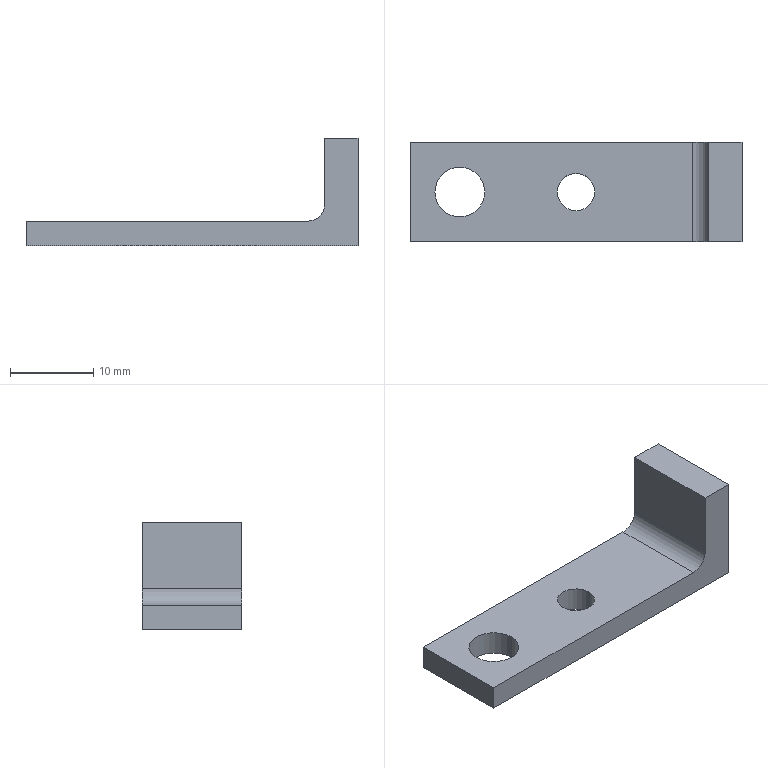Part | SolidWorks | features Extrusion 1, Fillet 1, ICE 1 | 1 solid | 13 faces | box 40 x 12 x 13 mm | volume 1798 mm3 | plane 8 | cylinder 5 | commonest cylinder face diameters 4.5 x2 6 x2 4 x1
STEP:
#1=CARTESIAN_POINT('',(3.,6.,3.));
#2=VERTEX_POINT('',#1);
#3=CARTESIAN_POINT('',(9.,6.,3.));
#4=VERTEX_POINT('',#3);
#5=CARTESIAN_POINT('',(6.,6.,3.));
#6=DIRECTION('',(0.,0.,1.));
#7=DIRECTION('',(1.,0.,0.));
#8=AXIS2_PLACEMENT_3D('',#5,#6,#7);
#9=CIRCLE('',#8,3.);
#10=EDGE_CURVE('',#2,#4,#9,.T.);
#11=ORIENTED_EDGE('',*,*,#10,.T.);
#12=CARTESIAN_POINT('',(9.,6.,0.));
#13=VERTEX_POINT('',#12);
#14=CARTESIAN_POINT('',(9.,6.,3.));
#15=DIRECTION('',(0.,0.,-1.));
#16=VECTOR('',#15,1000.);
#17=LINE('',#14,#16);
#18=EDGE_CURVE('',#4,#13,#17,.T.);
#19=ORIENTED_EDGE('',*,*,#18,.T.);
#20=CARTESIAN_POINT('',(3.,6.,0.));
#21=VERTEX_POINT('',#20);
#22=CARTESIAN_POINT('',(6.,6.,0.));
#23=DIRECTION('',(0.,0.,1.));
#24=DIRECTION('',(1.,0.,0.));
#25=AXIS2_PLACEMENT_3D('',#22,#23,#24);
#26=CIRCLE('',#25,3.);
#27=EDGE_CURVE('',#21,#13,#26,.T.);
#28=ORIENTED_EDGE('',*,*,#27,.F.);
#29=CARTESIAN_POINT('',(3.,6.,3.));
#30=DIRECTION('',(0.,0.,-1.));
#31=VECTOR('',#30,1000.);
#32=LINE('',#29,#31);
#33=EDGE_CURVE('',#2,#21,#32,.T.);
#34=ORIENTED_EDGE('',*,*,#33,.F.);
#35=EDGE_LOOP('',(#11,#19,#28,#34));
#36=FACE_OUTER_BOUND('',#35,.T.);
#37=CARTESIAN_POINT('',(6.,6.,3.));
#38=DIRECTION('',(0.,0.,-1.));
#39=DIRECTION('',(-1.,0.,0.));
#40=AXIS2_PLACEMENT_3D('',#37,#38,#39);
#41=CYLINDRICAL_SURFACE('',#40,3.);
#42=ADVANCED_FACE('',(#36),#41,.F.);
#43=CARTESIAN_POINT('',(17.75,6.,3.));
#44=VERTEX_POINT('',#43);
#45=CARTESIAN_POINT('',(22.25,6.,3.));
#46=VERTEX_POINT('',#45);
#47=CARTESIAN_POINT('',(20.,6.,3.));
#48=DIRECTION('',(0.,0.,1.));
#49=DIRECTION('',(1.,0.,0.));
#50=AXIS2_PLACEMENT_3D('',#47,#48,#49);
#51=CIRCLE('',#50,2.25);
#52=EDGE_CURVE('',#44,#46,#51,.T.);
#53=ORIENTED_EDGE('',*,*,#52,.T.);
#54=CARTESIAN_POINT('',(22.25,6.,0.));
#55=VERTEX_POINT('',#54);
#56=CARTESIAN_POINT('',(22.25,6.,3.));
#57=DIRECTION('',(0.,0.,-1.));
#58=VECTOR('',#57,1000.);
#59=LINE('',#56,#58);
#60=EDGE_CURVE('',#46,#55,#59,.T.);
#61=ORIENTED_EDGE('',*,*,#60,.T.);
#62=CARTESIAN_POINT('',(17.75,6.,0.));
#63=VERTEX_POINT('',#62);
#64=CARTESIAN_POINT('',(20.,6.,0.));
#65=DIRECTION('',(0.,0.,1.));
#66=DIRECTION('',(1.,0.,0.));
#67=AXIS2_PLACEMENT_3D('',#64,#65,#66);
#68=CIRCLE('',#67,2.25);
#69=EDGE_CURVE('',#63,#55,#68,.T.);
#70=ORIENTED_EDGE('',*,*,#69,.F.);
#71=CARTESIAN_POINT('',(17.75,6.,3.));
#72=DIRECTION('',(0.,0.,-1.));
#73=VECTOR('',#72,1000.);
#74=LINE('',#71,#73);
#75=EDGE_CURVE('',#44,#63,#74,.T.);
#76=ORIENTED_EDGE('',*,*,#75,.F.);
#77=EDGE_LOOP('',(#53,#61,#70,#76));
#78=FACE_OUTER_BOUND('',#77,.T.);
#79=CARTESIAN_POINT('',(20.,6.,3.));
#80=DIRECTION('',(0.,0.,-1.));
#81=DIRECTION('',(-1.,0.,0.));
#82=AXIS2_PLACEMENT_3D('',#79,#80,#81);
#83=CYLINDRICAL_SURFACE('',#82,2.25);
#84=ADVANCED_FACE('',(#78),#83,.F.);
#85=ORIENTED_EDGE('',*,*,#10,.F.);
#86=CARTESIAN_POINT('',(6.,6.,3.));
#87=DIRECTION('',(0.,0.,1.));
#88=DIRECTION('',(1.,0.,0.));
#89=AXIS2_PLACEMENT_3D('',#86,#87,#88);
#90=CIRCLE('',#89,3.);
#91=EDGE_CURVE('',#4,#2,#90,.T.);
#92=ORIENTED_EDGE('',*,*,#91,.F.);
#93=EDGE_LOOP('',(#85,#92));
#94=FACE_BOUND('',#93,.T.);
#95=ORIENTED_EDGE('',*,*,#52,.F.);
#96=CARTESIAN_POINT('',(20.,6.,3.));
#97=DIRECTION('',(0.,0.,1.));
#98=DIRECTION('',(1.,0.,0.));
#99=AXIS2_PLACEMENT_3D('',#96,#97,#98);
#100=CIRCLE('',#99,2.25);
#101=EDGE_CURVE('',#46,#44,#100,.T.);
#102=ORIENTED_EDGE('',*,*,#101,.F.);
#103=EDGE_LOOP('',(#95,#102));
#104=FACE_BOUND('',#103,.T.);
#105=CARTESIAN_POINT('',(0.,0.,3.));
#106=VERTEX_POINT('',#105);
#107=CARTESIAN_POINT('',(34.,0.,3.));
#108=VERTEX_POINT('',#107);
#109=CARTESIAN_POINT('',(0.,0.,3.));
#110=DIRECTION('',(1.,0.,0.));
#111=VECTOR('',#110,1000.);
#112=LINE('',#109,#111);
#113=EDGE_CURVE('',#106,#108,#112,.T.);
#114=ORIENTED_EDGE('',*,*,#113,.T.);
#115=CARTESIAN_POINT('',(34.,12.,3.));
#116=VERTEX_POINT('',#115);
#117=CARTESIAN_POINT('',(34.,12.,3.));
#118=DIRECTION('',(0.,1.,0.));
#119=VECTOR('',#118,1000.);
#120=LINE('',#117,#119);
#121=EDGE_CURVE('',#108,#116,#120,.T.);
#122=ORIENTED_EDGE('',*,*,#121,.T.);
#123=CARTESIAN_POINT('',(0.,12.,3.));
#124=VERTEX_POINT('',#123);
#125=CARTESIAN_POINT('',(0.,12.,3.));
#126=DIRECTION('',(-1.,0.,0.));
#127=VECTOR('',#126,1000.);
#128=LINE('',#125,#127);
#129=EDGE_CURVE('',#116,#124,#128,.T.);
#130=ORIENTED_EDGE('',*,*,#129,.T.);
#131=CARTESIAN_POINT('',(0.,0.,3.));
#132=DIRECTION('',(0.,-1.,0.));
#133=VECTOR('',#132,1000.);
#134=LINE('',#131,#133);
#135=EDGE_CURVE('',#124,#106,#134,.T.);
#136=ORIENTED_EDGE('',*,*,#135,.T.);
#137=EDGE_LOOP('',(#114,#122,#130,#136));
#138=FACE_OUTER_BOUND('',#137,.T.);
#139=CARTESIAN_POINT('',(0.,0.,3.));
#140=DIRECTION('',(0.,0.,-1.));
#141=DIRECTION('',(-1.,0.,0.));
#142=AXIS2_PLACEMENT_3D('',#139,#140,#141);
#143=PLANE('',#142);
#144=ADVANCED_FACE('',(#94,#104,#138),#143,.F.);
#145=ORIENTED_EDGE('',*,*,#69,.T.);
#146=CARTESIAN_POINT('',(20.,6.,0.));
#147=DIRECTION('',(0.,0.,1.));
#148=DIRECTION('',(1.,0.,0.));
#149=AXIS2_PLACEMENT_3D('',#146,#147,#148);
#150=CIRCLE('',#149,2.25);
#151=EDGE_CURVE('',#55,#63,#150,.T.);
#152=ORIENTED_EDGE('',*,*,#151,.T.);
#153=EDGE_LOOP('',(#145,#152));
#154=FACE_BOUND('',#153,.T.);
#155=CARTESIAN_POINT('',(0.,12.,0.));
#156=VERTEX_POINT('',#155);
#157=CARTESIAN_POINT('',(0.,0.,0.));
#158=VERTEX_POINT('',#157);
#159=CARTESIAN_POINT('',(0.,0.,0.));
#160=DIRECTION('',(0.,-1.,0.));
#161=VECTOR('',#160,1000.);
#162=LINE('',#159,#161);
#163=EDGE_CURVE('',#156,#158,#162,.T.);
#164=ORIENTED_EDGE('',*,*,#163,.F.);
#165=CARTESIAN_POINT('',(40.,12.,0.));
#166=VERTEX_POINT('',#165);
#167=CARTESIAN_POINT('',(0.,12.,0.));
#168=DIRECTION('',(-1.,0.,0.));
#169=VECTOR('',#168,1000.);
#170=LINE('',#167,#169);
#171=EDGE_CURVE('',#166,#156,#170,.T.);
#172=ORIENTED_EDGE('',*,*,#171,.F.);
#173=CARTESIAN_POINT('',(40.,0.,0.));
#174=VERTEX_POINT('',#173);
#175=CARTESIAN_POINT('',(40.,0.,0.));
#176=DIRECTION('',(0.,1.,0.));
#177=VECTOR('',#176,1000.);
#178=LINE('',#175,#177);
#179=EDGE_CURVE('',#174,#166,#178,.T.);
#180=ORIENTED_EDGE('',*,*,#179,.F.);
#181=CARTESIAN_POINT('',(0.,0.,0.));
#182=DIRECTION('',(1.,0.,0.));
#183=VECTOR('',#182,1000.);
#184=LINE('',#181,#183);
#185=EDGE_CURVE('',#158,#174,#184,.T.);
#186=ORIENTED_EDGE('',*,*,#185,.F.);
#187=EDGE_LOOP('',(#164,#172,#180,#186));
#188=FACE_OUTER_BOUND('',#187,.T.);
#189=ORIENTED_EDGE('',*,*,#27,.T.);
#190=CARTESIAN_POINT('',(6.,6.,0.));
#191=DIRECTION('',(0.,0.,1.));
#192=DIRECTION('',(1.,0.,0.));
#193=AXIS2_PLACEMENT_3D('',#190,#191,#192);
#194=CIRCLE('',#193,3.);
#195=EDGE_CURVE('',#13,#21,#194,.T.);
#196=ORIENTED_EDGE('',*,*,#195,.T.);
#197=EDGE_LOOP('',(#189,#196));
#198=FACE_BOUND('',#197,.T.);
#199=CARTESIAN_POINT('',(0.,0.,0.));
#200=DIRECTION('',(0.,0.,-1.));
#201=DIRECTION('',(-1.,0.,0.));
#202=AXIS2_PLACEMENT_3D('',#199,#200,#201);
#203=PLANE('',#202);
#204=ADVANCED_FACE('',(#154,#188,#198),#203,.T.);
#205=ORIENTED_EDGE('',*,*,#163,.T.);
#206=CARTESIAN_POINT('',(0.,0.,3.));
#207=DIRECTION('',(0.,0.,-1.));
#208=VECTOR('',#207,1000.);
#209=LINE('',#206,#208);
#210=EDGE_CURVE('',#106,#158,#209,.T.);
#211=ORIENTED_EDGE('',*,*,#210,.F.);
#212=ORIENTED_EDGE('',*,*,#135,.F.);
#213=CARTESIAN_POINT('',(0.,12.,3.));
#214=DIRECTION('',(0.,0.,-1.));
#215=VECTOR('',#214,1000.);
#216=LINE('',#213,#215);
#217=EDGE_CURVE('',#124,#156,#216,.T.);
#218=ORIENTED_EDGE('',*,*,#217,.T.);
#219=EDGE_LOOP('',(#205,#211,#212,#218));
#220=FACE_OUTER_BOUND('',#219,.T.);
#221=CARTESIAN_POINT('',(0.,0.,3.));
#222=DIRECTION('',(1.,0.,0.));
#223=DIRECTION('',(0.,0.,-1.));
#224=AXIS2_PLACEMENT_3D('',#221,#222,#223);
#225=PLANE('',#224);
#226=ADVANCED_FACE('',(#220),#225,.F.);
#227=ORIENTED_EDGE('',*,*,#185,.T.);
#228=CARTESIAN_POINT('',(40.,0.,13.));
#229=VERTEX_POINT('',#228);
#230=CARTESIAN_POINT('',(40.,0.,3.));
#231=DIRECTION('',(0.,0.,-1.));
#232=VECTOR('',#231,1000.);
#233=LINE('',#230,#232);
#234=EDGE_CURVE('',#229,#174,#233,.T.);
#235=ORIENTED_EDGE('',*,*,#234,.F.);
#236=CARTESIAN_POINT('',(36.,0.,13.));
#237=VERTEX_POINT('',#236);
#238=CARTESIAN_POINT('',(40.,0.,13.));
#239=DIRECTION('',(1.,0.,0.));
#240=VECTOR('',#239,1000.);
#241=LINE('',#238,#240);
#242=EDGE_CURVE('',#237,#229,#241,.T.);
#243=ORIENTED_EDGE('',*,*,#242,.F.);
#244=CARTESIAN_POINT('',(36.,0.,5.));
#245=VERTEX_POINT('',#244);
#246=CARTESIAN_POINT('',(36.,0.,13.));
#247=DIRECTION('',(0.,0.,-1.));
#248=VECTOR('',#247,1000.);
#249=LINE('',#246,#248);
#250=EDGE_CURVE('',#237,#245,#249,.T.);
#251=ORIENTED_EDGE('',*,*,#250,.T.);
#252=CARTESIAN_POINT('',(34.,0.,5.));
#253=DIRECTION('',(0.,1.,0.));
#254=DIRECTION('',(0.,0.,1.));
#255=AXIS2_PLACEMENT_3D('',#252,#253,#254);
#256=CIRCLE('',#255,2.);
#257=EDGE_CURVE('',#245,#108,#256,.T.);
#258=ORIENTED_EDGE('',*,*,#257,.T.);
#259=ORIENTED_EDGE('',*,*,#113,.F.);
#260=ORIENTED_EDGE('',*,*,#210,.T.);
#261=EDGE_LOOP('',(#227,#235,#243,#251,#258,#259,#260));
#262=FACE_OUTER_BOUND('',#261,.T.);
#263=CARTESIAN_POINT('',(0.,0.,3.));
#264=DIRECTION('',(0.,1.,0.));
#265=DIRECTION('',(0.,0.,1.));
#266=AXIS2_PLACEMENT_3D('',#263,#264,#265);
#267=PLANE('',#266);
#268=ADVANCED_FACE('',(#262),#267,.F.);
#269=ORIENTED_EDGE('',*,*,#179,.T.);
#270=CARTESIAN_POINT('',(40.,12.,13.));
#271=VERTEX_POINT('',#270);
#272=CARTESIAN_POINT('',(40.,12.,3.));
#273=DIRECTION('',(0.,0.,-1.));
#274=VECTOR('',#273,1000.);
#275=LINE('',#272,#274);
#276=EDGE_CURVE('',#271,#166,#275,.T.);
#277=ORIENTED_EDGE('',*,*,#276,.F.);
#278=CARTESIAN_POINT('',(40.,0.,13.));
#279=DIRECTION('',(0.,1.,0.));
#280=VECTOR('',#279,1000.);
#281=LINE('',#278,#280);
#282=EDGE_CURVE('',#229,#271,#281,.T.);
#283=ORIENTED_EDGE('',*,*,#282,.F.);
#284=ORIENTED_EDGE('',*,*,#234,.T.);
#285=EDGE_LOOP('',(#269,#277,#283,#284));
#286=FACE_OUTER_BOUND('',#285,.T.);
#287=CARTESIAN_POINT('',(40.,0.,3.));
#288=DIRECTION('',(-1.,0.,0.));
#289=DIRECTION('',(0.,0.,1.));
#290=AXIS2_PLACEMENT_3D('',#287,#288,#289);
#291=PLANE('',#290);
#292=ADVANCED_FACE('',(#286),#291,.F.);
#293=ORIENTED_EDGE('',*,*,#171,.T.);
#294=ORIENTED_EDGE('',*,*,#217,.F.);
#295=ORIENTED_EDGE('',*,*,#129,.F.);
#296=CARTESIAN_POINT('',(36.,12.,5.));
#297=VERTEX_POINT('',#296);
#298=CARTESIAN_POINT('',(34.,12.,5.));
#299=DIRECTION('',(0.,-1.,0.));
#300=DIRECTION('',(0.,0.,-1.));
#301=AXIS2_PLACEMENT_3D('',#298,#299,#300);
#302=CIRCLE('',#301,2.);
#303=EDGE_CURVE('',#116,#297,#302,.T.);
#304=ORIENTED_EDGE('',*,*,#303,.T.);
#305=CARTESIAN_POINT('',(36.,12.,13.));
#306=VERTEX_POINT('',#305);
#307=CARTESIAN_POINT('',(36.,12.,13.));
#308=DIRECTION('',(0.,0.,-1.));
#309=VECTOR('',#308,1000.);
#310=LINE('',#307,#309);
#311=EDGE_CURVE('',#306,#297,#310,.T.);
#312=ORIENTED_EDGE('',*,*,#311,.F.);
#313=CARTESIAN_POINT('',(40.,12.,13.));
#314=DIRECTION('',(-1.,0.,0.));
#315=VECTOR('',#314,1000.);
#316=LINE('',#313,#315);
#317=EDGE_CURVE('',#271,#306,#316,.T.);
#318=ORIENTED_EDGE('',*,*,#317,.F.);
#319=ORIENTED_EDGE('',*,*,#276,.T.);
#320=EDGE_LOOP('',(#293,#294,#295,#304,#312,#318,#319));
#321=FACE_OUTER_BOUND('',#320,.T.);
#322=CARTESIAN_POINT('',(0.,12.,3.));
#323=DIRECTION('',(0.,-1.,0.));
#324=DIRECTION('',(0.,0.,-1.));
#325=AXIS2_PLACEMENT_3D('',#322,#323,#324);
#326=PLANE('',#325);
#327=ADVANCED_FACE('',(#321),#326,.F.);
#328=ORIENTED_EDGE('',*,*,#60,.F.);
#329=ORIENTED_EDGE('',*,*,#101,.T.);
#330=ORIENTED_EDGE('',*,*,#75,.T.);
#331=ORIENTED_EDGE('',*,*,#151,.F.);
#332=EDGE_LOOP('',(#328,#329,#330,#331));
#333=FACE_OUTER_BOUND('',#332,.T.);
#334=CARTESIAN_POINT('',(20.,6.,3.));
#335=DIRECTION('',(0.,0.,-1.));
#336=DIRECTION('',(-1.,0.,0.));
#337=AXIS2_PLACEMENT_3D('',#334,#335,#336);
#338=CYLINDRICAL_SURFACE('',#337,2.25);
#339=ADVANCED_FACE('',(#333),#338,.F.);
#340=ORIENTED_EDGE('',*,*,#18,.F.);
#341=ORIENTED_EDGE('',*,*,#91,.T.);
#342=ORIENTED_EDGE('',*,*,#33,.T.);
#343=ORIENTED_EDGE('',*,*,#195,.F.);
#344=EDGE_LOOP('',(#340,#341,#342,#343));
#345=FACE_OUTER_BOUND('',#344,.T.);
#346=CARTESIAN_POINT('',(6.,6.,3.));
#347=DIRECTION('',(0.,0.,-1.));
#348=DIRECTION('',(-1.,0.,0.));
#349=AXIS2_PLACEMENT_3D('',#346,#347,#348);
#350=CYLINDRICAL_SURFACE('',#349,3.);
#351=ADVANCED_FACE('',(#345),#350,.F.);
#352=ORIENTED_EDGE('',*,*,#311,.T.);
#353=CARTESIAN_POINT('',(36.,0.,5.));
#354=DIRECTION('',(0.,-1.,0.));
#355=VECTOR('',#354,1000.);
#356=LINE('',#353,#355);
#357=EDGE_CURVE('',#297,#245,#356,.T.);
#358=ORIENTED_EDGE('',*,*,#357,.T.);
#359=ORIENTED_EDGE('',*,*,#250,.F.);
#360=CARTESIAN_POINT('',(36.,0.,13.));
#361=DIRECTION('',(0.,-1.,0.));
#362=VECTOR('',#361,1000.);
#363=LINE('',#360,#362);
#364=EDGE_CURVE('',#306,#237,#363,.T.);
#365=ORIENTED_EDGE('',*,*,#364,.F.);
#366=EDGE_LOOP('',(#352,#358,#359,#365));
#367=FACE_OUTER_BOUND('',#366,.T.);
#368=CARTESIAN_POINT('',(36.,0.,13.));
#369=DIRECTION('',(1.,0.,0.));
#370=DIRECTION('',(0.,0.,-1.));
#371=AXIS2_PLACEMENT_3D('',#368,#369,#370);
#372=PLANE('',#371);
#373=ADVANCED_FACE('',(#367),#372,.F.);
#374=ORIENTED_EDGE('',*,*,#282,.T.);
#375=ORIENTED_EDGE('',*,*,#317,.T.);
#376=ORIENTED_EDGE('',*,*,#364,.T.);
#377=ORIENTED_EDGE('',*,*,#242,.T.);
#378=EDGE_LOOP('',(#374,#375,#376,#377));
#379=FACE_OUTER_BOUND('',#378,.T.);
#380=CARTESIAN_POINT('',(0.,0.,13.));
#381=DIRECTION('',(0.,0.,1.));
#382=DIRECTION('',(1.,0.,0.));
#383=AXIS2_PLACEMENT_3D('',#380,#381,#382);
#384=PLANE('',#383);
#385=ADVANCED_FACE('',(#379),#384,.T.);
#386=ORIENTED_EDGE('',*,*,#303,.F.);
#387=ORIENTED_EDGE('',*,*,#121,.F.);
#388=ORIENTED_EDGE('',*,*,#257,.F.);
#389=ORIENTED_EDGE('',*,*,#357,.F.);
#390=EDGE_LOOP('',(#386,#387,#388,#389));
#391=FACE_OUTER_BOUND('',#390,.T.);
#392=CARTESIAN_POINT('',(34.,0.,5.));
#393=DIRECTION('',(0.,1.,0.));
#394=DIRECTION('',(0.,0.,1.));
#395=AXIS2_PLACEMENT_3D('',#392,#393,#394);
#396=CYLINDRICAL_SURFACE('',#395,2.);
#397=ADVANCED_FACE('',(#391),#396,.F.);
#398=CLOSED_SHELL('',(#42,#84,#144,#204,#226,#268,#292,#327,#339,#351,#373,#385,#397));
#399=MANIFOLD_SOLID_BREP('',#398);
#400=CARTESIAN_POINT('',(0.,0.,0.));
#401=DIRECTION('',(0.,0.,1.));
#402=DIRECTION('',(1.,0.,0.));
#403=AXIS2_PLACEMENT_3D('',#400,#401,#402);
#404=(LENGTH_UNIT()NAMED_UNIT(*)SI_UNIT(.MILLI.,.METRE.));
#405=UNCERTAINTY_MEASURE_WITH_UNIT(LENGTH_MEASURE(0.00001),#404,'','');
#406=(NAMED_UNIT(*)PLANE_ANGLE_UNIT()SI_UNIT($,.RADIAN.));
#407=(NAMED_UNIT(*)SI_UNIT($,.STERADIAN.)SOLID_ANGLE_UNIT());
#408=(GEOMETRIC_REPRESENTATION_CONTEXT(3)GLOBAL_UNCERTAINTY_ASSIGNED_CONTEXT((#405))GLOBAL_UNIT_ASSIGNED_CONTEXT((#404,#406,#407))REPRESENTATION_CONTEXT('',''));
#409=ADVANCED_BREP_SHAPE_REPRESENTATION('',(#399,#403),#408);